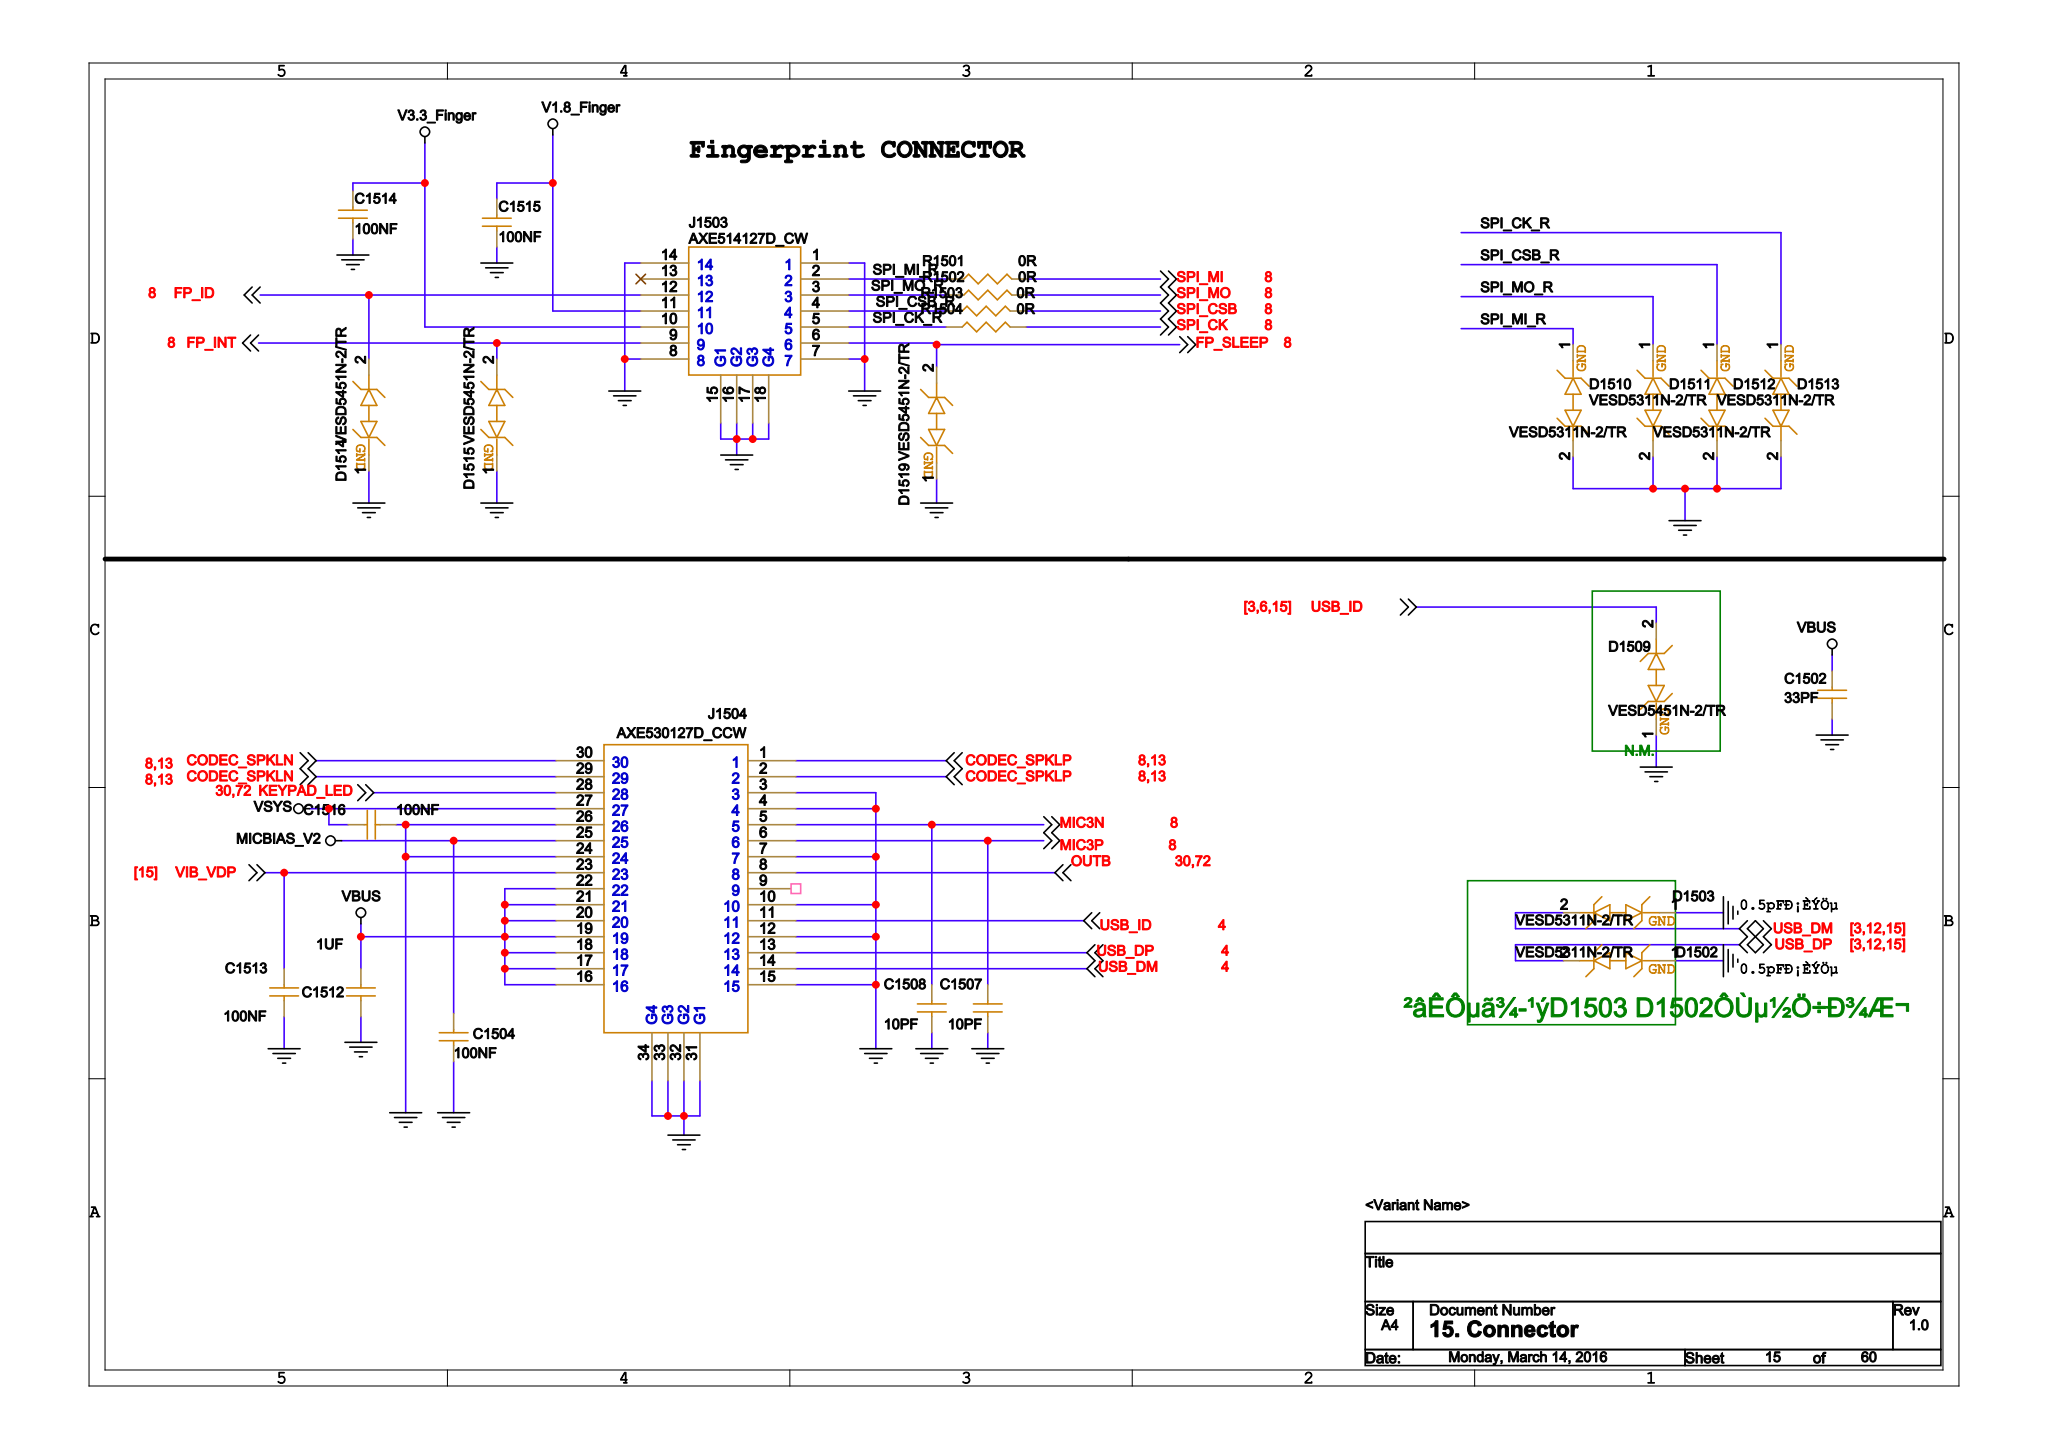Circuit board | Cadence Allegro | 1088 parts | 793 nets | one sheet of the schematic
Parts on this sheet (reference | value | footprint):
C1502 | 33PF | C0201
C1504 | 100NF | C0201
C1507 | 10PF | C0201
C1508 | 10PF | C0201
C1512 | 1UF | C0201
C1513 | 100NF | C0201
C1514 | 100NF | C0201
C1515 | 100NF | C0201
C1516 | 100NF | C0201
D1503 | VESD5311N-2/TR | DFN1006-2
D1509
D1510 | VESD5311N-2/TR | DFN1006-2
D1511 | VESD5311N-2/TR | DFN1006-2
D1512 | VESD5311N-2/TR | DFN1006-2
D1513 | VESD5311N-2/TR | DFN1006-2
J1503 | AXE514127D_CW | BTB_AXE514124_CW
J1504 | AXE530127D_CCW | BTB_AXE530124_CCW
R1501 | 0R | R0201
R1502 | 0R | R0201
R1503 | 0R | R0201
R1504 | 0R | R0201
Nets of these parts (net: part-pin ...):
GND: C1502-2 C1504-2 C1507-2 C1508-2 C1512-2 C1513-2 C1514-2 C1515-2 C1516-2 D1503-1 D1509-1 D1510-2 D1511-2 D1512-2 D1513-2 J1503-1 J1503-7 J1503-8 J1503-14 J1503-15 J1503-16 J1503-17 J1503-18 J1504-3 J1504-4 J1504-7 J1504-10 J1504-12 J1504-15 J1504-24 J1504-26 J1504-31 J1504-32 J1504-33 J1504-34
OUTB: J1504-8
VSYS: C1516-1 J1504-27
MICBIAS_V2: C1504-1 J1504-25
FP_SLEEP: J1503-6
FP_INT: J1503-9
FP_ID: J1503-12
USB_ID: D1509-2 J1504-11
SPI_CK: R1504-2
SPI_CSB: R1503-2
SPI_MI: R1501-2
SPI_MO: R1502-2
USB_DM: D1503-2 J1504-14
USB_DP: J1504-13
CODEC_SPKLP: J1504-1 J1504-2
CODEC_SPKLN: J1504-29 J1504-30
V3.3_FINGER: C1514-1 J1503-10
VBUS: C1502-1 C1512-1 J1504-16 J1504-17 J1504-18 J1504-19 J1504-20 J1504-21 J1504-22
V1.8_FINGER: C1515-1 J1503-11
MIC3P: C1507-1 J1504-6
MIC3N: C1508-1 J1504-5
VIB_VDP: C1513-1 J1504-23
SPI_MI_R: D1510-1 J1503-2 R1501-1
SPI_MO_R: D1511-1 J1503-3 R1502-1
SPI_CSB_R: D1512-1 J1503-4 R1503-1
SPI_CK_R: D1513-1 J1503-5 R1504-1
KEYPAD_LED: J1504-28